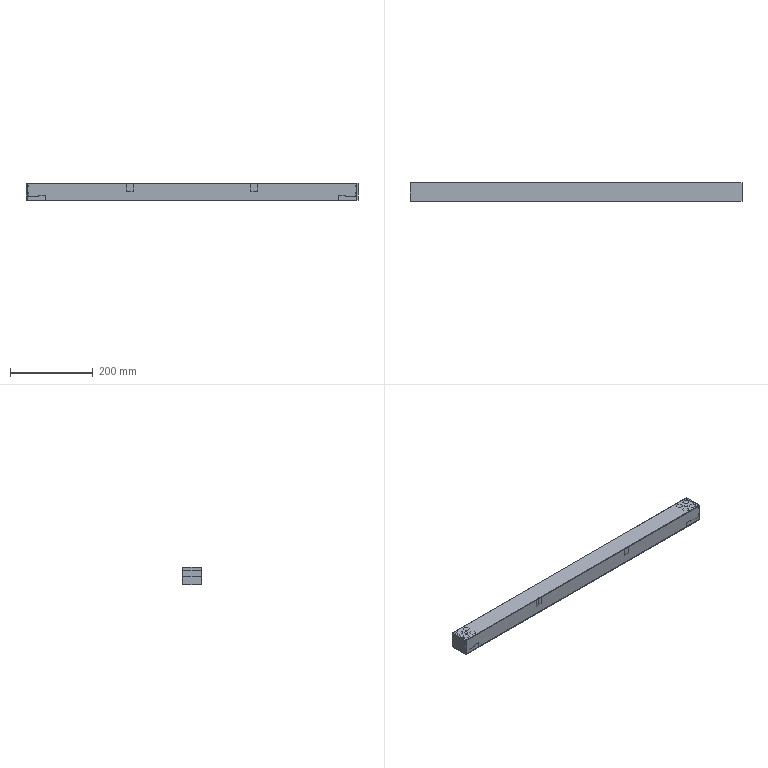Part | 4 solids | 90 faces | box 801.8 x 45 x 42 mm | volume 5745420 mm3 | plane 50 | cylinder 40 | commonest cylinder face diameters 8.5 x16 14 x16 8 x4 34 x4